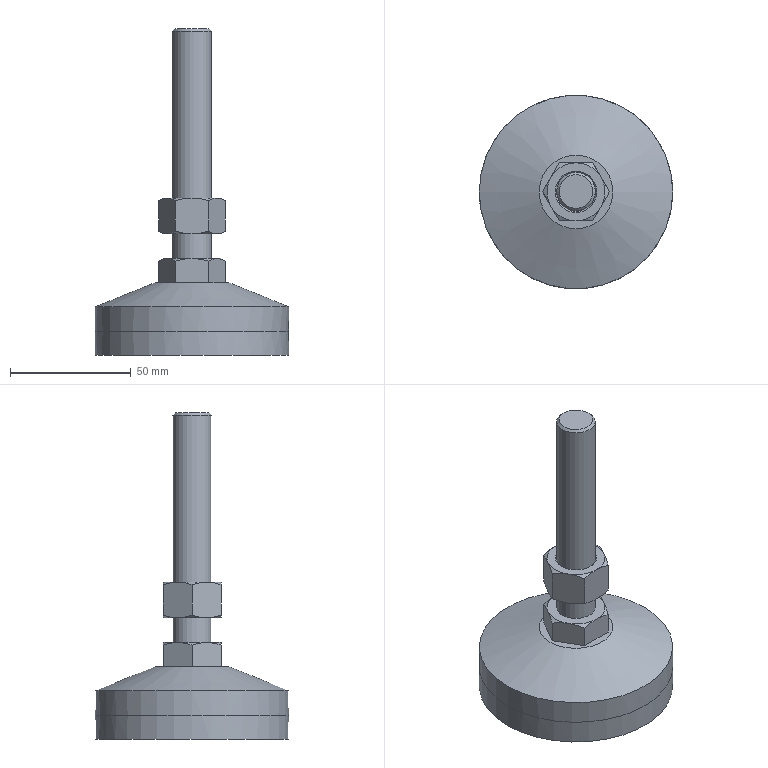Part | STEP file | Foot cup | 1 solid | 44 faces | box 80 x 80 x 135 mm | volume 154518 mm3 | cone 22 | plane 18 | cylinder 4 | commonest cylinder face diameters 16 x2 80 x2